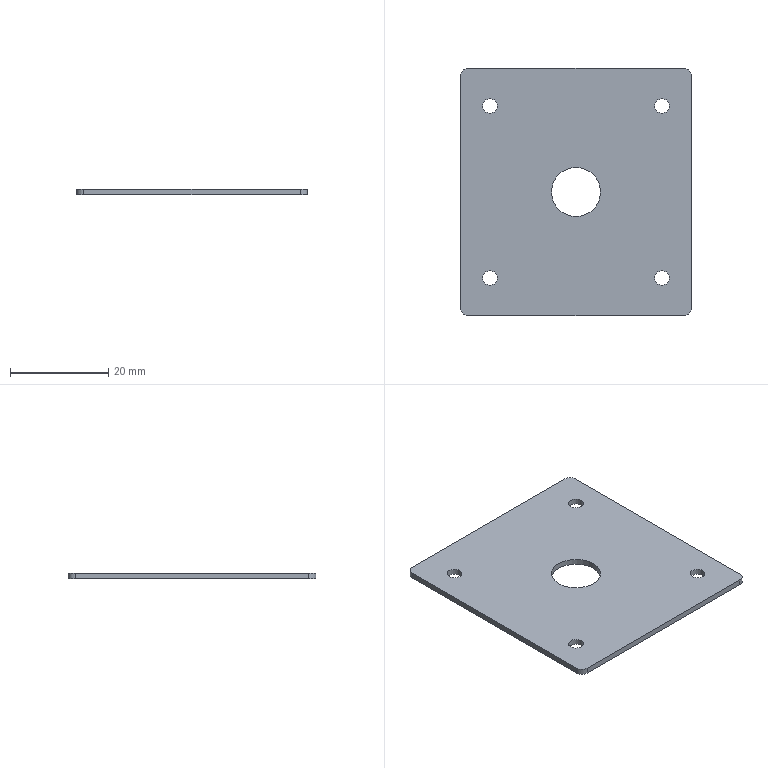Part | NX | features DATUM_CSYS 2, EXTRUDE 1, SKETCH 1 | 1 solid | 15 faces | box 47 x 50.372 x 1.2 mm | volume 2711 mm3 | cylinder 9 | plane 6 | commonest cylinder face diameters 3 x8 10 x1
STEP:
#1=CARTESIAN_POINT('',(-23.5,-23.686,0.));
#2=VERTEX_POINT('',#1);
#3=CARTESIAN_POINT('',(-23.5,23.686,0.));
#4=VERTEX_POINT('',#3);
#5=CARTESIAN_POINT('',(-23.5,-23.686,0.));
#6=DIRECTION('',(0.,1.,0.));
#7=VECTOR('',#6,1000.);
#8=LINE('',#5,#7);
#9=EDGE_CURVE('',#2,#4,#8,.T.);
#10=ORIENTED_EDGE('',*,*,#9,.F.);
#11=CARTESIAN_POINT('',(-23.5,-23.686,1.2));
#12=VERTEX_POINT('',#11);
#13=CARTESIAN_POINT('',(-23.5,-23.686,1.2));
#14=DIRECTION('',(0.,0.,-1.));
#15=VECTOR('',#14,1000.);
#16=LINE('',#13,#15);
#17=EDGE_CURVE('',#12,#2,#16,.T.);
#18=ORIENTED_EDGE('',*,*,#17,.F.);
#19=CARTESIAN_POINT('',(-23.5,23.686,1.2));
#20=VERTEX_POINT('',#19);
#21=CARTESIAN_POINT('',(-23.5,-23.686,1.2));
#22=DIRECTION('',(0.,1.,0.));
#23=VECTOR('',#22,1000.);
#24=LINE('',#21,#23);
#25=EDGE_CURVE('',#12,#20,#24,.T.);
#26=ORIENTED_EDGE('',*,*,#25,.T.);
#27=CARTESIAN_POINT('',(-23.5,23.686,1.2));
#28=DIRECTION('',(0.,0.,-1.));
#29=VECTOR('',#28,1000.);
#30=LINE('',#27,#29);
#31=EDGE_CURVE('',#20,#4,#30,.T.);
#32=ORIENTED_EDGE('',*,*,#31,.T.);
#33=EDGE_LOOP('',(#10,#18,#26,#32));
#34=FACE_BOUND('',#33,.T.);
#35=CARTESIAN_POINT('',(-23.5,-23.686,1.2));
#36=DIRECTION('',(-1.,0.,0.));
#37=DIRECTION('',(0.,0.,1.));
#38=AXIS2_PLACEMENT_3D('',#35,#36,#37);
#39=PLANE('',#38);
#40=ADVANCED_FACE('',(#34),#39,.T.);
#41=CARTESIAN_POINT('',(-22.,25.186,0.));
#42=VERTEX_POINT('',#41);
#43=CARTESIAN_POINT('',(-22.,23.686,0.));
#44=DIRECTION('',(0.,0.,-1.));
#45=DIRECTION('',(1.,0.,0.));
#46=AXIS2_PLACEMENT_3D('',#43,#44,#45);
#47=CIRCLE('',#46,1.5);
#48=EDGE_CURVE('',#4,#42,#47,.T.);
#49=ORIENTED_EDGE('',*,*,#48,.F.);
#50=ORIENTED_EDGE('',*,*,#31,.F.);
#51=CARTESIAN_POINT('',(-22.,25.186,1.2));
#52=VERTEX_POINT('',#51);
#53=CARTESIAN_POINT('',(-22.,23.686,1.2));
#54=DIRECTION('',(0.,0.,-1.));
#55=DIRECTION('',(1.,0.,0.));
#56=AXIS2_PLACEMENT_3D('',#53,#54,#55);
#57=CIRCLE('',#56,1.5);
#58=EDGE_CURVE('',#20,#52,#57,.T.);
#59=ORIENTED_EDGE('',*,*,#58,.T.);
#60=CARTESIAN_POINT('',(-22.,25.186,1.2));
#61=DIRECTION('',(0.,0.,-1.));
#62=VECTOR('',#61,1000.);
#63=LINE('',#60,#62);
#64=EDGE_CURVE('',#52,#42,#63,.T.);
#65=ORIENTED_EDGE('',*,*,#64,.T.);
#66=EDGE_LOOP('',(#49,#50,#59,#65));
#67=FACE_BOUND('',#66,.T.);
#68=CARTESIAN_POINT('',(-22.,23.686,1.2));
#69=DIRECTION('',(0.,0.,-1.));
#70=DIRECTION('',(-1.,0.,0.));
#71=AXIS2_PLACEMENT_3D('',#68,#69,#70);
#72=CYLINDRICAL_SURFACE('',#71,1.5);
#73=ADVANCED_FACE('',(#67),#72,.T.);
#74=CARTESIAN_POINT('',(22.,25.186,0.));
#75=VERTEX_POINT('',#74);
#76=CARTESIAN_POINT('',(-22.,25.186,0.));
#77=DIRECTION('',(1.,0.,0.));
#78=VECTOR('',#77,1000.);
#79=LINE('',#76,#78);
#80=EDGE_CURVE('',#42,#75,#79,.T.);
#81=ORIENTED_EDGE('',*,*,#80,.F.);
#82=ORIENTED_EDGE('',*,*,#64,.F.);
#83=CARTESIAN_POINT('',(22.,25.186,1.2));
#84=VERTEX_POINT('',#83);
#85=CARTESIAN_POINT('',(-22.,25.186,1.2));
#86=DIRECTION('',(1.,0.,0.));
#87=VECTOR('',#86,1000.);
#88=LINE('',#85,#87);
#89=EDGE_CURVE('',#52,#84,#88,.T.);
#90=ORIENTED_EDGE('',*,*,#89,.T.);
#91=CARTESIAN_POINT('',(22.,25.186,1.2));
#92=DIRECTION('',(0.,0.,-1.));
#93=VECTOR('',#92,1000.);
#94=LINE('',#91,#93);
#95=EDGE_CURVE('',#84,#75,#94,.T.);
#96=ORIENTED_EDGE('',*,*,#95,.T.);
#97=EDGE_LOOP('',(#81,#82,#90,#96));
#98=FACE_BOUND('',#97,.T.);
#99=CARTESIAN_POINT('',(-22.,25.186,1.2));
#100=DIRECTION('',(0.,1.,0.));
#101=DIRECTION('',(0.,0.,1.));
#102=AXIS2_PLACEMENT_3D('',#99,#100,#101);
#103=PLANE('',#102);
#104=ADVANCED_FACE('',(#98),#103,.T.);
#105=CARTESIAN_POINT('',(23.5,23.686,0.));
#106=VERTEX_POINT('',#105);
#107=CARTESIAN_POINT('',(22.,23.686,0.));
#108=DIRECTION('',(0.,0.,-1.));
#109=DIRECTION('',(1.,0.,0.));
#110=AXIS2_PLACEMENT_3D('',#107,#108,#109);
#111=CIRCLE('',#110,1.5);
#112=EDGE_CURVE('',#75,#106,#111,.T.);
#113=ORIENTED_EDGE('',*,*,#112,.F.);
#114=ORIENTED_EDGE('',*,*,#95,.F.);
#115=CARTESIAN_POINT('',(23.5,23.686,1.2));
#116=VERTEX_POINT('',#115);
#117=CARTESIAN_POINT('',(22.,23.686,1.2));
#118=DIRECTION('',(0.,0.,-1.));
#119=DIRECTION('',(1.,0.,0.));
#120=AXIS2_PLACEMENT_3D('',#117,#118,#119);
#121=CIRCLE('',#120,1.5);
#122=EDGE_CURVE('',#84,#116,#121,.T.);
#123=ORIENTED_EDGE('',*,*,#122,.T.);
#124=CARTESIAN_POINT('',(23.5,23.686,1.2));
#125=DIRECTION('',(0.,0.,-1.));
#126=VECTOR('',#125,1000.);
#127=LINE('',#124,#126);
#128=EDGE_CURVE('',#116,#106,#127,.T.);
#129=ORIENTED_EDGE('',*,*,#128,.T.);
#130=EDGE_LOOP('',(#113,#114,#123,#129));
#131=FACE_BOUND('',#130,.T.);
#132=CARTESIAN_POINT('',(22.,23.686,1.2));
#133=DIRECTION('',(0.,0.,-1.));
#134=DIRECTION('',(-1.,0.,0.));
#135=AXIS2_PLACEMENT_3D('',#132,#133,#134);
#136=CYLINDRICAL_SURFACE('',#135,1.5);
#137=ADVANCED_FACE('',(#131),#136,.T.);
#138=CARTESIAN_POINT('',(23.5,-23.686,0.));
#139=VERTEX_POINT('',#138);
#140=CARTESIAN_POINT('',(23.5,23.686,0.));
#141=DIRECTION('',(0.,-1.,0.));
#142=VECTOR('',#141,1000.);
#143=LINE('',#140,#142);
#144=EDGE_CURVE('',#106,#139,#143,.T.);
#145=ORIENTED_EDGE('',*,*,#144,.F.);
#146=ORIENTED_EDGE('',*,*,#128,.F.);
#147=CARTESIAN_POINT('',(23.5,-23.686,1.2));
#148=VERTEX_POINT('',#147);
#149=CARTESIAN_POINT('',(23.5,23.686,1.2));
#150=DIRECTION('',(0.,-1.,0.));
#151=VECTOR('',#150,1000.);
#152=LINE('',#149,#151);
#153=EDGE_CURVE('',#116,#148,#152,.T.);
#154=ORIENTED_EDGE('',*,*,#153,.T.);
#155=CARTESIAN_POINT('',(23.5,-23.686,1.2));
#156=DIRECTION('',(0.,0.,-1.));
#157=VECTOR('',#156,1000.);
#158=LINE('',#155,#157);
#159=EDGE_CURVE('',#148,#139,#158,.T.);
#160=ORIENTED_EDGE('',*,*,#159,.T.);
#161=EDGE_LOOP('',(#145,#146,#154,#160));
#162=FACE_BOUND('',#161,.T.);
#163=CARTESIAN_POINT('',(23.5,23.686,1.2));
#164=DIRECTION('',(1.,0.,0.));
#165=DIRECTION('',(0.,0.,-1.));
#166=AXIS2_PLACEMENT_3D('',#163,#164,#165);
#167=PLANE('',#166);
#168=ADVANCED_FACE('',(#162),#167,.T.);
#169=CARTESIAN_POINT('',(22.,-25.186,0.));
#170=VERTEX_POINT('',#169);
#171=CARTESIAN_POINT('',(22.,-23.686,0.));
#172=DIRECTION('',(0.,0.,-1.));
#173=DIRECTION('',(1.,0.,0.));
#174=AXIS2_PLACEMENT_3D('',#171,#172,#173);
#175=CIRCLE('',#174,1.5);
#176=EDGE_CURVE('',#139,#170,#175,.T.);
#177=ORIENTED_EDGE('',*,*,#176,.F.);
#178=ORIENTED_EDGE('',*,*,#159,.F.);
#179=CARTESIAN_POINT('',(22.,-25.186,1.2));
#180=VERTEX_POINT('',#179);
#181=CARTESIAN_POINT('',(22.,-23.686,1.2));
#182=DIRECTION('',(0.,0.,-1.));
#183=DIRECTION('',(1.,0.,0.));
#184=AXIS2_PLACEMENT_3D('',#181,#182,#183);
#185=CIRCLE('',#184,1.5);
#186=EDGE_CURVE('',#148,#180,#185,.T.);
#187=ORIENTED_EDGE('',*,*,#186,.T.);
#188=CARTESIAN_POINT('',(22.,-25.186,1.2));
#189=DIRECTION('',(0.,0.,-1.));
#190=VECTOR('',#189,1000.);
#191=LINE('',#188,#190);
#192=EDGE_CURVE('',#180,#170,#191,.T.);
#193=ORIENTED_EDGE('',*,*,#192,.T.);
#194=EDGE_LOOP('',(#177,#178,#187,#193));
#195=FACE_BOUND('',#194,.T.);
#196=CARTESIAN_POINT('',(22.,-23.686,1.2));
#197=DIRECTION('',(0.,0.,-1.));
#198=DIRECTION('',(-1.,0.,0.));
#199=AXIS2_PLACEMENT_3D('',#196,#197,#198);
#200=CYLINDRICAL_SURFACE('',#199,1.5);
#201=ADVANCED_FACE('',(#195),#200,.T.);
#202=CARTESIAN_POINT('',(-22.,-25.186,0.));
#203=VERTEX_POINT('',#202);
#204=CARTESIAN_POINT('',(22.,-25.186,0.));
#205=DIRECTION('',(-1.,0.,0.));
#206=VECTOR('',#205,1000.);
#207=LINE('',#204,#206);
#208=EDGE_CURVE('',#170,#203,#207,.T.);
#209=ORIENTED_EDGE('',*,*,#208,.F.);
#210=ORIENTED_EDGE('',*,*,#192,.F.);
#211=CARTESIAN_POINT('',(-22.,-25.186,1.2));
#212=VERTEX_POINT('',#211);
#213=CARTESIAN_POINT('',(22.,-25.186,1.2));
#214=DIRECTION('',(-1.,0.,0.));
#215=VECTOR('',#214,1000.);
#216=LINE('',#213,#215);
#217=EDGE_CURVE('',#180,#212,#216,.T.);
#218=ORIENTED_EDGE('',*,*,#217,.T.);
#219=CARTESIAN_POINT('',(-22.,-25.186,1.2));
#220=DIRECTION('',(0.,0.,-1.));
#221=VECTOR('',#220,1000.);
#222=LINE('',#219,#221);
#223=EDGE_CURVE('',#212,#203,#222,.T.);
#224=ORIENTED_EDGE('',*,*,#223,.T.);
#225=EDGE_LOOP('',(#209,#210,#218,#224));
#226=FACE_BOUND('',#225,.T.);
#227=CARTESIAN_POINT('',(22.,-25.186,1.2));
#228=DIRECTION('',(0.,-1.,0.));
#229=DIRECTION('',(0.,0.,-1.));
#230=AXIS2_PLACEMENT_3D('',#227,#228,#229);
#231=PLANE('',#230);
#232=ADVANCED_FACE('',(#226),#231,.T.);
#233=CARTESIAN_POINT('',(-16.,17.5,1.2));
#234=VERTEX_POINT('',#233);
#235=CARTESIAN_POINT('',(-17.5,17.5,1.2));
#236=DIRECTION('',(0.,0.,1.));
#237=DIRECTION('',(1.,0.,0.));
#238=AXIS2_PLACEMENT_3D('',#235,#236,#237);
#239=CIRCLE('',#238,1.5);
#240=EDGE_CURVE('',#234,#234,#239,.T.);
#241=ORIENTED_EDGE('',*,*,#240,.T.);
#242=EDGE_LOOP('',(#241));
#243=FACE_BOUND('',#242,.T.);
#244=CARTESIAN_POINT('',(-16.,17.5,0.));
#245=VERTEX_POINT('',#244);
#246=CARTESIAN_POINT('',(-17.5,17.5,0.));
#247=DIRECTION('',(0.,0.,1.));
#248=DIRECTION('',(1.,0.,0.));
#249=AXIS2_PLACEMENT_3D('',#246,#247,#248);
#250=CIRCLE('',#249,1.5);
#251=EDGE_CURVE('',#245,#245,#250,.T.);
#252=ORIENTED_EDGE('',*,*,#251,.F.);
#253=EDGE_LOOP('',(#252));
#254=FACE_BOUND('',#253,.T.);
#255=CARTESIAN_POINT('',(-17.5,17.5,1.2));
#256=DIRECTION('',(0.,0.,-1.));
#257=DIRECTION('',(-1.,0.,0.));
#258=AXIS2_PLACEMENT_3D('',#255,#256,#257);
#259=CYLINDRICAL_SURFACE('',#258,1.5);
#260=ADVANCED_FACE('',(#243,#254),#259,.F.);
#261=CARTESIAN_POINT('',(5.,0.,1.2));
#262=VERTEX_POINT('',#261);
#263=CARTESIAN_POINT('',(0.,0.,1.2));
#264=DIRECTION('',(0.,0.,1.));
#265=DIRECTION('',(1.,0.,0.));
#266=AXIS2_PLACEMENT_3D('',#263,#264,#265);
#267=CIRCLE('',#266,5.);
#268=EDGE_CURVE('',#262,#262,#267,.T.);
#269=ORIENTED_EDGE('',*,*,#268,.T.);
#270=EDGE_LOOP('',(#269));
#271=FACE_BOUND('',#270,.T.);
#272=CARTESIAN_POINT('',(5.,0.,0.));
#273=VERTEX_POINT('',#272);
#274=CARTESIAN_POINT('',(0.,0.,0.));
#275=DIRECTION('',(0.,0.,1.));
#276=DIRECTION('',(1.,0.,0.));
#277=AXIS2_PLACEMENT_3D('',#274,#275,#276);
#278=CIRCLE('',#277,5.);
#279=EDGE_CURVE('',#273,#273,#278,.T.);
#280=ORIENTED_EDGE('',*,*,#279,.F.);
#281=EDGE_LOOP('',(#280));
#282=FACE_BOUND('',#281,.T.);
#283=CARTESIAN_POINT('',(0.,0.,1.2));
#284=DIRECTION('',(0.,0.,-1.));
#285=DIRECTION('',(-1.,0.,0.));
#286=AXIS2_PLACEMENT_3D('',#283,#284,#285);
#287=CYLINDRICAL_SURFACE('',#286,5.);
#288=ADVANCED_FACE('',(#271,#282),#287,.F.);
#289=CARTESIAN_POINT('',(19.,-17.5,1.2));
#290=VERTEX_POINT('',#289);
#291=CARTESIAN_POINT('',(17.5,-17.5,1.2));
#292=DIRECTION('',(0.,0.,1.));
#293=DIRECTION('',(1.,0.,0.));
#294=AXIS2_PLACEMENT_3D('',#291,#292,#293);
#295=CIRCLE('',#294,1.5);
#296=EDGE_CURVE('',#290,#290,#295,.T.);
#297=ORIENTED_EDGE('',*,*,#296,.T.);
#298=EDGE_LOOP('',(#297));
#299=FACE_BOUND('',#298,.T.);
#300=CARTESIAN_POINT('',(19.,-17.5,0.));
#301=VERTEX_POINT('',#300);
#302=CARTESIAN_POINT('',(17.5,-17.5,0.));
#303=DIRECTION('',(0.,0.,1.));
#304=DIRECTION('',(1.,0.,0.));
#305=AXIS2_PLACEMENT_3D('',#302,#303,#304);
#306=CIRCLE('',#305,1.5);
#307=EDGE_CURVE('',#301,#301,#306,.T.);
#308=ORIENTED_EDGE('',*,*,#307,.F.);
#309=EDGE_LOOP('',(#308));
#310=FACE_BOUND('',#309,.T.);
#311=CARTESIAN_POINT('',(17.5,-17.5,1.2));
#312=DIRECTION('',(0.,0.,-1.));
#313=DIRECTION('',(-1.,0.,0.));
#314=AXIS2_PLACEMENT_3D('',#311,#312,#313);
#315=CYLINDRICAL_SURFACE('',#314,1.5);
#316=ADVANCED_FACE('',(#299,#310),#315,.F.);
#317=CARTESIAN_POINT('',(19.,17.5,1.2));
#318=VERTEX_POINT('',#317);
#319=CARTESIAN_POINT('',(17.5,17.5,1.2));
#320=DIRECTION('',(0.,0.,1.));
#321=DIRECTION('',(1.,0.,0.));
#322=AXIS2_PLACEMENT_3D('',#319,#320,#321);
#323=CIRCLE('',#322,1.5);
#324=EDGE_CURVE('',#318,#318,#323,.T.);
#325=ORIENTED_EDGE('',*,*,#324,.T.);
#326=EDGE_LOOP('',(#325));
#327=FACE_BOUND('',#326,.T.);
#328=CARTESIAN_POINT('',(19.,17.5,0.));
#329=VERTEX_POINT('',#328);
#330=CARTESIAN_POINT('',(17.5,17.5,0.));
#331=DIRECTION('',(0.,0.,1.));
#332=DIRECTION('',(1.,0.,0.));
#333=AXIS2_PLACEMENT_3D('',#330,#331,#332);
#334=CIRCLE('',#333,1.5);
#335=EDGE_CURVE('',#329,#329,#334,.T.);
#336=ORIENTED_EDGE('',*,*,#335,.F.);
#337=EDGE_LOOP('',(#336));
#338=FACE_BOUND('',#337,.T.);
#339=CARTESIAN_POINT('',(17.5,17.5,1.2));
#340=DIRECTION('',(0.,0.,-1.));
#341=DIRECTION('',(-1.,0.,0.));
#342=AXIS2_PLACEMENT_3D('',#339,#340,#341);
#343=CYLINDRICAL_SURFACE('',#342,1.5);
#344=ADVANCED_FACE('',(#327,#338),#343,.F.);
#345=CARTESIAN_POINT('',(-22.,-23.686,0.));
#346=DIRECTION('',(0.,0.,-1.));
#347=DIRECTION('',(1.,0.,0.));
#348=AXIS2_PLACEMENT_3D('',#345,#346,#347);
#349=CIRCLE('',#348,1.5);
#350=EDGE_CURVE('',#203,#2,#349,.T.);
#351=ORIENTED_EDGE('',*,*,#350,.F.);
#352=ORIENTED_EDGE('',*,*,#223,.F.);
#353=CARTESIAN_POINT('',(-22.,-23.686,1.2));
#354=DIRECTION('',(0.,0.,-1.));
#355=DIRECTION('',(1.,0.,0.));
#356=AXIS2_PLACEMENT_3D('',#353,#354,#355);
#357=CIRCLE('',#356,1.5);
#358=EDGE_CURVE('',#212,#12,#357,.T.);
#359=ORIENTED_EDGE('',*,*,#358,.T.);
#360=ORIENTED_EDGE('',*,*,#17,.T.);
#361=EDGE_LOOP('',(#351,#352,#359,#360));
#362=FACE_BOUND('',#361,.T.);
#363=CARTESIAN_POINT('',(-22.,-23.686,1.2));
#364=DIRECTION('',(0.,0.,-1.));
#365=DIRECTION('',(-1.,0.,0.));
#366=AXIS2_PLACEMENT_3D('',#363,#364,#365);
#367=CYLINDRICAL_SURFACE('',#366,1.5);
#368=ADVANCED_FACE('',(#362),#367,.T.);
#369=CARTESIAN_POINT('',(-16.,-17.5,1.2));
#370=VERTEX_POINT('',#369);
#371=CARTESIAN_POINT('',(-17.5,-17.5,1.2));
#372=DIRECTION('',(0.,0.,1.));
#373=DIRECTION('',(1.,0.,0.));
#374=AXIS2_PLACEMENT_3D('',#371,#372,#373);
#375=CIRCLE('',#374,1.5);
#376=EDGE_CURVE('',#370,#370,#375,.T.);
#377=ORIENTED_EDGE('',*,*,#376,.T.);
#378=EDGE_LOOP('',(#377));
#379=FACE_BOUND('',#378,.T.);
#380=CARTESIAN_POINT('',(-16.,-17.5,0.));
#381=VERTEX_POINT('',#380);
#382=CARTESIAN_POINT('',(-17.5,-17.5,0.));
#383=DIRECTION('',(0.,0.,1.));
#384=DIRECTION('',(1.,0.,0.));
#385=AXIS2_PLACEMENT_3D('',#382,#383,#384);
#386=CIRCLE('',#385,1.5);
#387=EDGE_CURVE('',#381,#381,#386,.T.);
#388=ORIENTED_EDGE('',*,*,#387,.F.);
#389=EDGE_LOOP('',(#388));
#390=FACE_BOUND('',#389,.T.);
#391=CARTESIAN_POINT('',(-17.5,-17.5,1.2));
#392=DIRECTION('',(0.,0.,-1.));
#393=DIRECTION('',(-1.,0.,0.));
#394=AXIS2_PLACEMENT_3D('',#391,#392,#393);
#395=CYLINDRICAL_SURFACE('',#394,1.5);
#396=ADVANCED_FACE('',(#379,#390),#395,.F.);
#397=ORIENTED_EDGE('',*,*,#25,.F.);
#398=ORIENTED_EDGE('',*,*,#358,.F.);
#399=ORIENTED_EDGE('',*,*,#217,.F.);
#400=ORIENTED_EDGE('',*,*,#186,.F.);
#401=ORIENTED_EDGE('',*,*,#153,.F.);
#402=ORIENTED_EDGE('',*,*,#122,.F.);
#403=ORIENTED_EDGE('',*,*,#89,.F.);
#404=ORIENTED_EDGE('',*,*,#58,.F.);
#405=EDGE_LOOP('',(#397,#398,#399,#400,#401,#402,#403,#404));
#406=FACE_BOUND('',#405,.T.);
#407=ORIENTED_EDGE('',*,*,#324,.F.);
#408=EDGE_LOOP('',(#407));
#409=FACE_BOUND('',#408,.T.);
#410=ORIENTED_EDGE('',*,*,#296,.F.);
#411=EDGE_LOOP('',(#410));
#412=FACE_BOUND('',#411,.T.);
#413=ORIENTED_EDGE('',*,*,#268,.F.);
#414=EDGE_LOOP('',(#413));
#415=FACE_BOUND('',#414,.T.);
#416=ORIENTED_EDGE('',*,*,#240,.F.);
#417=EDGE_LOOP('',(#416));
#418=FACE_BOUND('',#417,.T.);
#419=ORIENTED_EDGE('',*,*,#376,.F.);
#420=EDGE_LOOP('',(#419));
#421=FACE_BOUND('',#420,.T.);
#422=CARTESIAN_POINT('',(-22.,23.686,1.2));
#423=DIRECTION('',(0.,0.,-1.));
#424=DIRECTION('',(-1.,0.,0.));
#425=AXIS2_PLACEMENT_3D('',#422,#423,#424);
#426=PLANE('',#425);
#427=ADVANCED_FACE('',(#406,#409,#412,#415,#418,#421),#426,.F.);
#428=ORIENTED_EDGE('',*,*,#9,.T.);
#429=ORIENTED_EDGE('',*,*,#48,.T.);
#430=ORIENTED_EDGE('',*,*,#80,.T.);
#431=ORIENTED_EDGE('',*,*,#112,.T.);
#432=ORIENTED_EDGE('',*,*,#144,.T.);
#433=ORIENTED_EDGE('',*,*,#176,.T.);
#434=ORIENTED_EDGE('',*,*,#208,.T.);
#435=ORIENTED_EDGE('',*,*,#350,.T.);
#436=EDGE_LOOP('',(#428,#429,#430,#431,#432,#433,#434,#435));
#437=FACE_BOUND('',#436,.T.);
#438=ORIENTED_EDGE('',*,*,#335,.T.);
#439=EDGE_LOOP('',(#438));
#440=FACE_BOUND('',#439,.T.);
#441=ORIENTED_EDGE('',*,*,#307,.T.);
#442=EDGE_LOOP('',(#441));
#443=FACE_BOUND('',#442,.T.);
#444=ORIENTED_EDGE('',*,*,#279,.T.);
#445=EDGE_LOOP('',(#444));
#446=FACE_BOUND('',#445,.T.);
#447=ORIENTED_EDGE('',*,*,#251,.T.);
#448=EDGE_LOOP('',(#447));
#449=FACE_BOUND('',#448,.T.);
#450=ORIENTED_EDGE('',*,*,#387,.T.);
#451=EDGE_LOOP('',(#450));
#452=FACE_BOUND('',#451,.T.);
#453=CARTESIAN_POINT('',(-22.,23.686,0.));
#454=DIRECTION('',(0.,0.,-1.));
#455=DIRECTION('',(-1.,0.,0.));
#456=AXIS2_PLACEMENT_3D('',#453,#454,#455);
#457=PLANE('',#456);
#458=ADVANCED_FACE('',(#437,#440,#443,#446,#449,#452),#457,.T.);
#459=CLOSED_SHELL('',(#40,#73,#104,#137,#168,#201,#232,#260,#288,#316,#344,#368,#396,#427,#458));
#460=MANIFOLD_SOLID_BREP('',#459);
#461=(LENGTH_UNIT()NAMED_UNIT(*)SI_UNIT(.MILLI.,.METRE.));
#462=UNCERTAINTY_MEASURE_WITH_UNIT(LENGTH_MEASURE(0.00001),#461,'','');
#463=(NAMED_UNIT(*)PLANE_ANGLE_UNIT()SI_UNIT($,.RADIAN.));
#464=(NAMED_UNIT(*)SI_UNIT($,.STERADIAN.)SOLID_ANGLE_UNIT());
#465=(GEOMETRIC_REPRESENTATION_CONTEXT(3)GLOBAL_UNCERTAINTY_ASSIGNED_CONTEXT((#462))GLOBAL_UNIT_ASSIGNED_CONTEXT((#461,#463,#464))REPRESENTATION_CONTEXT('',''));
#466=ADVANCED_BREP_SHAPE_REPRESENTATION('',(#460),#465);